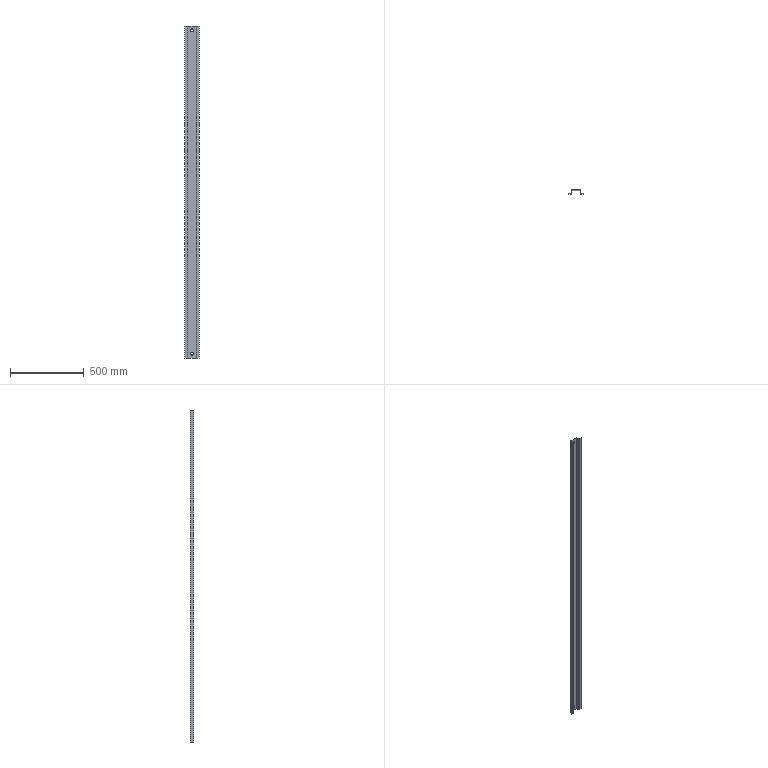Part | 1 solid | 42 faces | box 98.4 x 25 x 2251 mm | volume 259526 mm3 | plane 30 | cylinder 12 | commonest cylinder face diameters 2 x4 3.6 x4 20 x4
STEP:
#1=CARTESIAN_POINT('',(10.,-0.8,-1095.5));
#2=VERTEX_POINT('',#1);
#3=CARTESIAN_POINT('',(-10.,-0.8,-1095.5));
#4=VERTEX_POINT('',#3);
#5=CARTESIAN_POINT('',(0.,-0.8,-1095.5));
#6=DIRECTION('',(0.,1.,0.));
#7=DIRECTION('',(-1.,0.,0.));
#8=AXIS2_PLACEMENT_3D('',#5,#6,#7);
#9=CIRCLE('',#8,10.);
#10=EDGE_CURVE('',#2,#4,#9,.T.);
#11=ORIENTED_EDGE('',*,*,#10,.F.);
#12=CARTESIAN_POINT('',(10.,0.,-1095.5));
#13=VERTEX_POINT('',#12);
#14=CARTESIAN_POINT('',(10.,-10.,-1095.5));
#15=DIRECTION('',(0.,1.,0.));
#16=VECTOR('',#15,1000.);
#17=LINE('',#14,#16);
#18=EDGE_CURVE('',#2,#13,#17,.T.);
#19=ORIENTED_EDGE('',*,*,#18,.T.);
#20=CARTESIAN_POINT('',(-10.,0.,-1095.5));
#21=VERTEX_POINT('',#20);
#22=CARTESIAN_POINT('',(0.,0.,-1095.5));
#23=DIRECTION('',(0.,1.,0.));
#24=DIRECTION('',(-1.,0.,0.));
#25=AXIS2_PLACEMENT_3D('',#22,#23,#24);
#26=CIRCLE('',#25,10.);
#27=EDGE_CURVE('',#13,#21,#26,.T.);
#28=ORIENTED_EDGE('',*,*,#27,.T.);
#29=CARTESIAN_POINT('',(-10.,-10.,-1095.5));
#30=DIRECTION('',(0.,1.,0.));
#31=VECTOR('',#30,1000.);
#32=LINE('',#29,#31);
#33=EDGE_CURVE('',#4,#21,#32,.T.);
#34=ORIENTED_EDGE('',*,*,#33,.F.);
#35=EDGE_LOOP('',(#11,#19,#28,#34));
#36=FACE_OUTER_BOUND('',#35,.T.);
#37=CARTESIAN_POINT('',(0.,-10.,-1095.5));
#38=DIRECTION('',(0.,1.,0.));
#39=DIRECTION('',(-1.,0.,0.));
#40=AXIS2_PLACEMENT_3D('',#37,#38,#39);
#41=CYLINDRICAL_SURFACE('',#40,10.);
#42=ADVANCED_FACE('',(#36),#41,.F.);
#43=CARTESIAN_POINT('',(10.,-0.8,1095.5));
#44=VERTEX_POINT('',#43);
#45=CARTESIAN_POINT('',(-10.,-0.8,1095.5));
#46=VERTEX_POINT('',#45);
#47=CARTESIAN_POINT('',(0.,-0.8,1095.5));
#48=DIRECTION('',(0.,1.,0.));
#49=DIRECTION('',(-1.,0.,0.));
#50=AXIS2_PLACEMENT_3D('',#47,#48,#49);
#51=CIRCLE('',#50,10.);
#52=EDGE_CURVE('',#44,#46,#51,.T.);
#53=ORIENTED_EDGE('',*,*,#52,.F.);
#54=CARTESIAN_POINT('',(10.,0.,1095.5));
#55=VERTEX_POINT('',#54);
#56=CARTESIAN_POINT('',(10.,-10.,1095.5));
#57=DIRECTION('',(0.,1.,0.));
#58=VECTOR('',#57,1000.);
#59=LINE('',#56,#58);
#60=EDGE_CURVE('',#44,#55,#59,.T.);
#61=ORIENTED_EDGE('',*,*,#60,.T.);
#62=CARTESIAN_POINT('',(-10.,0.,1095.5));
#63=VERTEX_POINT('',#62);
#64=CARTESIAN_POINT('',(0.,0.,1095.5));
#65=DIRECTION('',(0.,1.,0.));
#66=DIRECTION('',(1.,0.,0.));
#67=AXIS2_PLACEMENT_3D('',#64,#65,#66);
#68=CIRCLE('',#67,10.);
#69=EDGE_CURVE('',#55,#63,#68,.T.);
#70=ORIENTED_EDGE('',*,*,#69,.T.);
#71=CARTESIAN_POINT('',(-10.,-10.,1095.5));
#72=DIRECTION('',(0.,1.,0.));
#73=VECTOR('',#72,1000.);
#74=LINE('',#71,#73);
#75=EDGE_CURVE('',#46,#63,#74,.T.);
#76=ORIENTED_EDGE('',*,*,#75,.F.);
#77=EDGE_LOOP('',(#53,#61,#70,#76));
#78=FACE_OUTER_BOUND('',#77,.T.);
#79=CARTESIAN_POINT('',(0.,-10.,1095.5));
#80=DIRECTION('',(0.,1.,0.));
#81=DIRECTION('',(-1.,0.,0.));
#82=AXIS2_PLACEMENT_3D('',#79,#80,#81);
#83=CYLINDRICAL_SURFACE('',#82,10.);
#84=ADVANCED_FACE('',(#78),#83,.F.);
#85=CARTESIAN_POINT('',(29.2,-23.2,-1125.5));
#86=VERTEX_POINT('',#85);
#87=CARTESIAN_POINT('',(29.2,-23.2,1125.5));
#88=VERTEX_POINT('',#87);
#89=CARTESIAN_POINT('',(29.2,-23.2,-1125.5));
#90=DIRECTION('',(0.,0.,1.));
#91=VECTOR('',#90,1000.);
#92=LINE('',#89,#91);
#93=EDGE_CURVE('',#86,#88,#92,.T.);
#94=ORIENTED_EDGE('',*,*,#93,.T.);
#95=CARTESIAN_POINT('',(29.2,-1.8,1125.5));
#96=VERTEX_POINT('',#95);
#97=CARTESIAN_POINT('',(29.2,0.,1125.5));
#98=DIRECTION('',(0.,-1.,0.));
#99=VECTOR('',#98,1000.);
#100=LINE('',#97,#99);
#101=EDGE_CURVE('',#96,#88,#100,.T.);
#102=ORIENTED_EDGE('',*,*,#101,.F.);
#103=CARTESIAN_POINT('',(29.2,-1.8,-1125.5));
#104=VERTEX_POINT('',#103);
#105=CARTESIAN_POINT('',(29.2,-1.8,1125.5));
#106=DIRECTION('',(0.,0.,-1.));
#107=VECTOR('',#106,1000.);
#108=LINE('',#105,#107);
#109=EDGE_CURVE('',#96,#104,#108,.T.);
#110=ORIENTED_EDGE('',*,*,#109,.T.);
#111=CARTESIAN_POINT('',(29.2,0.,-1125.5));
#112=DIRECTION('',(0.,-1.,0.));
#113=VECTOR('',#112,1000.);
#114=LINE('',#111,#113);
#115=EDGE_CURVE('',#104,#86,#114,.T.);
#116=ORIENTED_EDGE('',*,*,#115,.T.);
#117=EDGE_LOOP('',(#94,#102,#110,#116));
#118=FACE_OUTER_BOUND('',#117,.T.);
#119=CARTESIAN_POINT('',(29.2,0.,1125.5));
#120=DIRECTION('',(1.,0.,0.));
#121=DIRECTION('',(0.,1.,0.));
#122=AXIS2_PLACEMENT_3D('',#119,#120,#121);
#123=PLANE('',#122);
#124=ADVANCED_FACE('',(#118),#123,.F.);
#125=CARTESIAN_POINT('',(30.,-1.8,1125.5));
#126=VERTEX_POINT('',#125);
#127=CARTESIAN_POINT('',(30.,-23.2,1125.5));
#128=VERTEX_POINT('',#127);
#129=CARTESIAN_POINT('',(30.,0.,1125.5));
#130=DIRECTION('',(0.,-1.,0.));
#131=VECTOR('',#130,1000.);
#132=LINE('',#129,#131);
#133=EDGE_CURVE('',#126,#128,#132,.T.);
#134=ORIENTED_EDGE('',*,*,#133,.T.);
#135=CARTESIAN_POINT('',(30.,-23.2,-1125.5));
#136=VERTEX_POINT('',#135);
#137=CARTESIAN_POINT('',(30.,-23.2,-1125.5));
#138=DIRECTION('',(0.,0.,1.));
#139=VECTOR('',#138,1000.);
#140=LINE('',#137,#139);
#141=EDGE_CURVE('',#136,#128,#140,.T.);
#142=ORIENTED_EDGE('',*,*,#141,.F.);
#143=CARTESIAN_POINT('',(30.,-1.8,-1125.5));
#144=VERTEX_POINT('',#143);
#145=CARTESIAN_POINT('',(30.,0.,-1125.5));
#146=DIRECTION('',(0.,-1.,0.));
#147=VECTOR('',#146,1000.);
#148=LINE('',#145,#147);
#149=EDGE_CURVE('',#144,#136,#148,.T.);
#150=ORIENTED_EDGE('',*,*,#149,.F.);
#151=CARTESIAN_POINT('',(30.,-1.8,1125.5));
#152=DIRECTION('',(0.,0.,-1.));
#153=VECTOR('',#152,1000.);
#154=LINE('',#151,#153);
#155=EDGE_CURVE('',#126,#144,#154,.T.);
#156=ORIENTED_EDGE('',*,*,#155,.F.);
#157=EDGE_LOOP('',(#134,#142,#150,#156));
#158=FACE_OUTER_BOUND('',#157,.T.);
#159=CARTESIAN_POINT('',(30.,0.,1125.5));
#160=DIRECTION('',(1.,0.,0.));
#161=DIRECTION('',(0.,1.,0.));
#162=AXIS2_PLACEMENT_3D('',#159,#160,#161);
#163=PLANE('',#162);
#164=ADVANCED_FACE('',(#158),#163,.T.);
#165=CARTESIAN_POINT('',(30.,-23.2,-1125.5));
#166=DIRECTION('',(-1.,0.,0.));
#167=VECTOR('',#166,1000.);
#168=LINE('',#165,#167);
#169=EDGE_CURVE('',#136,#86,#168,.T.);
#170=ORIENTED_EDGE('',*,*,#169,.T.);
#171=ORIENTED_EDGE('',*,*,#115,.F.);
#172=CARTESIAN_POINT('',(29.2,-1.8,-1125.5));
#173=DIRECTION('',(1.,0.,0.));
#174=VECTOR('',#173,1000.);
#175=LINE('',#172,#174);
#176=EDGE_CURVE('',#104,#144,#175,.T.);
#177=ORIENTED_EDGE('',*,*,#176,.T.);
#178=ORIENTED_EDGE('',*,*,#149,.T.);
#179=EDGE_LOOP('',(#170,#171,#177,#178));
#180=FACE_OUTER_BOUND('',#179,.T.);
#181=CARTESIAN_POINT('',(28.2,-1.8,-1125.5));
#182=DIRECTION('',(0.,0.,1.));
#183=DIRECTION('',(1.,0.,0.));
#184=AXIS2_PLACEMENT_3D('',#181,#182,#183);
#185=PLANE('',#184);
#186=ADVANCED_FACE('',(#180),#185,.F.);
#187=CARTESIAN_POINT('',(-30.,-23.2,-1125.5));
#188=VERTEX_POINT('',#187);
#189=CARTESIAN_POINT('',(-30.,-1.8,-1125.5));
#190=VERTEX_POINT('',#189);
#191=CARTESIAN_POINT('',(-30.,-25.,-1125.5));
#192=DIRECTION('',(0.,1.,0.));
#193=VECTOR('',#192,1000.);
#194=LINE('',#191,#193);
#195=EDGE_CURVE('',#188,#190,#194,.T.);
#196=ORIENTED_EDGE('',*,*,#195,.F.);
#197=CARTESIAN_POINT('',(-30.,-23.2,1125.5));
#198=VERTEX_POINT('',#197);
#199=CARTESIAN_POINT('',(-30.,-23.2,1125.5));
#200=DIRECTION('',(0.,0.,-1.));
#201=VECTOR('',#200,1000.);
#202=LINE('',#199,#201);
#203=EDGE_CURVE('',#198,#188,#202,.T.);
#204=ORIENTED_EDGE('',*,*,#203,.F.);
#205=CARTESIAN_POINT('',(-30.,-1.8,1125.5));
#206=VERTEX_POINT('',#205);
#207=CARTESIAN_POINT('',(-30.,-25.,1125.5));
#208=DIRECTION('',(0.,1.,0.));
#209=VECTOR('',#208,1000.);
#210=LINE('',#207,#209);
#211=EDGE_CURVE('',#198,#206,#210,.T.);
#212=ORIENTED_EDGE('',*,*,#211,.T.);
#213=CARTESIAN_POINT('',(-30.,-1.8,1125.5));
#214=DIRECTION('',(0.,0.,-1.));
#215=VECTOR('',#214,1000.);
#216=LINE('',#213,#215);
#217=EDGE_CURVE('',#206,#190,#216,.T.);
#218=ORIENTED_EDGE('',*,*,#217,.T.);
#219=EDGE_LOOP('',(#196,#204,#212,#218));
#220=FACE_OUTER_BOUND('',#219,.T.);
#221=CARTESIAN_POINT('',(-30.,-25.,1125.5));
#222=DIRECTION('',(-1.,0.,0.));
#223=DIRECTION('',(0.,0.,1.));
#224=AXIS2_PLACEMENT_3D('',#221,#222,#223);
#225=PLANE('',#224);
#226=ADVANCED_FACE('',(#220),#225,.T.);
#227=CARTESIAN_POINT('',(-29.2,-23.2,1125.5));
#228=VERTEX_POINT('',#227);
#229=CARTESIAN_POINT('',(-29.2,-23.2,-1125.5));
#230=VERTEX_POINT('',#229);
#231=CARTESIAN_POINT('',(-29.2,-23.2,1125.5));
#232=DIRECTION('',(0.,0.,-1.));
#233=VECTOR('',#232,1000.);
#234=LINE('',#231,#233);
#235=EDGE_CURVE('',#228,#230,#234,.T.);
#236=ORIENTED_EDGE('',*,*,#235,.T.);
#237=CARTESIAN_POINT('',(-29.2,-1.8,-1125.5));
#238=VERTEX_POINT('',#237);
#239=CARTESIAN_POINT('',(-29.2,-25.,-1125.5));
#240=DIRECTION('',(0.,1.,0.));
#241=VECTOR('',#240,1000.);
#242=LINE('',#239,#241);
#243=EDGE_CURVE('',#230,#238,#242,.T.);
#244=ORIENTED_EDGE('',*,*,#243,.T.);
#245=CARTESIAN_POINT('',(-29.2,-1.8,1125.5));
#246=VERTEX_POINT('',#245);
#247=CARTESIAN_POINT('',(-29.2,-1.8,1125.5));
#248=DIRECTION('',(0.,0.,-1.));
#249=VECTOR('',#248,1000.);
#250=LINE('',#247,#249);
#251=EDGE_CURVE('',#246,#238,#250,.T.);
#252=ORIENTED_EDGE('',*,*,#251,.F.);
#253=CARTESIAN_POINT('',(-29.2,-25.,1125.5));
#254=DIRECTION('',(0.,1.,0.));
#255=VECTOR('',#254,1000.);
#256=LINE('',#253,#255);
#257=EDGE_CURVE('',#228,#246,#256,.T.);
#258=ORIENTED_EDGE('',*,*,#257,.F.);
#259=EDGE_LOOP('',(#236,#244,#252,#258));
#260=FACE_OUTER_BOUND('',#259,.T.);
#261=CARTESIAN_POINT('',(-29.2,-25.,1125.5));
#262=DIRECTION('',(-1.,0.,0.));
#263=DIRECTION('',(0.,0.,1.));
#264=AXIS2_PLACEMENT_3D('',#261,#262,#263);
#265=PLANE('',#264);
#266=ADVANCED_FACE('',(#260),#265,.F.);
#267=ORIENTED_EDGE('',*,*,#211,.F.);
#268=CARTESIAN_POINT('',(-30.,-23.2,1125.5));
#269=DIRECTION('',(1.,0.,0.));
#270=VECTOR('',#269,1000.);
#271=LINE('',#268,#270);
#272=EDGE_CURVE('',#198,#228,#271,.T.);
#273=ORIENTED_EDGE('',*,*,#272,.T.);
#274=ORIENTED_EDGE('',*,*,#257,.T.);
#275=CARTESIAN_POINT('',(-29.2,-1.8,1125.5));
#276=DIRECTION('',(-1.,0.,0.));
#277=VECTOR('',#276,1000.);
#278=LINE('',#275,#277);
#279=EDGE_CURVE('',#246,#206,#278,.T.);
#280=ORIENTED_EDGE('',*,*,#279,.T.);
#281=EDGE_LOOP('',(#267,#273,#274,#280));
#282=FACE_OUTER_BOUND('',#281,.T.);
#283=CARTESIAN_POINT('',(28.2,-1.8,1125.5));
#284=DIRECTION('',(0.,0.,1.));
#285=DIRECTION('',(1.,0.,0.));
#286=AXIS2_PLACEMENT_3D('',#283,#284,#285);
#287=PLANE('',#286);
#288=ADVANCED_FACE('',(#282),#287,.T.);
#289=CARTESIAN_POINT('',(-28.2,0.,1125.5));
#290=VERTEX_POINT('',#289);
#291=CARTESIAN_POINT('',(-28.2,-0.8,1125.5));
#292=VERTEX_POINT('',#291);
#293=CARTESIAN_POINT('',(-28.2,0.,1125.5));
#294=DIRECTION('',(0.,-1.,0.));
#295=VECTOR('',#294,1000.);
#296=LINE('',#293,#295);
#297=EDGE_CURVE('',#290,#292,#296,.T.);
#298=ORIENTED_EDGE('',*,*,#297,.F.);
#299=CARTESIAN_POINT('',(-28.2,-1.8,1125.5));
#300=DIRECTION('',(0.,0.,-1.));
#301=DIRECTION('',(1.,0.,0.));
#302=AXIS2_PLACEMENT_3D('',#299,#300,#301);
#303=CIRCLE('',#302,1.8);
#304=EDGE_CURVE('',#206,#290,#303,.T.);
#305=ORIENTED_EDGE('',*,*,#304,.F.);
#306=ORIENTED_EDGE('',*,*,#279,.F.);
#307=CARTESIAN_POINT('',(-28.2,-1.8,1125.5));
#308=DIRECTION('',(0.,0.,-1.));
#309=DIRECTION('',(1.,0.,0.));
#310=AXIS2_PLACEMENT_3D('',#307,#308,#309);
#311=CIRCLE('',#310,1.);
#312=EDGE_CURVE('',#246,#292,#311,.T.);
#313=ORIENTED_EDGE('',*,*,#312,.T.);
#314=EDGE_LOOP('',(#298,#305,#306,#313));
#315=FACE_OUTER_BOUND('',#314,.T.);
#316=CARTESIAN_POINT('',(-28.2,0.,1125.5));
#317=DIRECTION('',(0.,0.,1.));
#318=DIRECTION('',(1.,0.,0.));
#319=AXIS2_PLACEMENT_3D('',#316,#317,#318);
#320=PLANE('',#319);
#321=ADVANCED_FACE('',(#315),#320,.T.);
#322=CARTESIAN_POINT('',(28.2,0.,1125.5));
#323=VERTEX_POINT('',#322);
#324=CARTESIAN_POINT('',(-30.,0.,1125.5));
#325=DIRECTION('',(1.,0.,0.));
#326=VECTOR('',#325,1000.);
#327=LINE('',#324,#326);
#328=EDGE_CURVE('',#290,#323,#327,.T.);
#329=ORIENTED_EDGE('',*,*,#328,.F.);
#330=ORIENTED_EDGE('',*,*,#297,.T.);
#331=CARTESIAN_POINT('',(28.2,-0.8,1125.5));
#332=VERTEX_POINT('',#331);
#333=CARTESIAN_POINT('',(-30.,-0.8,1125.5));
#334=DIRECTION('',(1.,0.,0.));
#335=VECTOR('',#334,1000.);
#336=LINE('',#333,#335);
#337=EDGE_CURVE('',#292,#332,#336,.T.);
#338=ORIENTED_EDGE('',*,*,#337,.T.);
#339=CARTESIAN_POINT('',(28.2,-0.8,1125.5));
#340=DIRECTION('',(0.,1.,0.));
#341=VECTOR('',#340,1000.);
#342=LINE('',#339,#341);
#343=EDGE_CURVE('',#332,#323,#342,.T.);
#344=ORIENTED_EDGE('',*,*,#343,.T.);
#345=EDGE_LOOP('',(#329,#330,#338,#344));
#346=FACE_OUTER_BOUND('',#345,.T.);
#347=CARTESIAN_POINT('',(-29.2,-1.8,1125.5));
#348=DIRECTION('',(0.,0.,1.));
#349=DIRECTION('',(1.,0.,0.));
#350=AXIS2_PLACEMENT_3D('',#347,#348,#349);
#351=PLANE('',#350);
#352=ADVANCED_FACE('',(#346),#351,.T.);
#353=CARTESIAN_POINT('',(-30.,-1.8,-1125.5));
#354=DIRECTION('',(1.,0.,0.));
#355=VECTOR('',#354,1000.);
#356=LINE('',#353,#355);
#357=EDGE_CURVE('',#190,#238,#356,.T.);
#358=ORIENTED_EDGE('',*,*,#357,.F.);
#359=CARTESIAN_POINT('',(-28.2,0.,-1125.5));
#360=VERTEX_POINT('',#359);
#361=CARTESIAN_POINT('',(-28.2,-1.8,-1125.5));
#362=DIRECTION('',(0.,0.,-1.));
#363=DIRECTION('',(1.,0.,0.));
#364=AXIS2_PLACEMENT_3D('',#361,#362,#363);
#365=CIRCLE('',#364,1.8);
#366=EDGE_CURVE('',#190,#360,#365,.T.);
#367=ORIENTED_EDGE('',*,*,#366,.T.);
#368=CARTESIAN_POINT('',(-28.2,-0.8,-1125.5));
#369=VERTEX_POINT('',#368);
#370=CARTESIAN_POINT('',(-28.2,-0.8,-1125.5));
#371=DIRECTION('',(0.,1.,0.));
#372=VECTOR('',#371,1000.);
#373=LINE('',#370,#372);
#374=EDGE_CURVE('',#369,#360,#373,.T.);
#375=ORIENTED_EDGE('',*,*,#374,.F.);
#376=CARTESIAN_POINT('',(-28.2,-1.8,-1125.5));
#377=DIRECTION('',(0.,0.,-1.));
#378=DIRECTION('',(1.,0.,0.));
#379=AXIS2_PLACEMENT_3D('',#376,#377,#378);
#380=CIRCLE('',#379,1.);
#381=EDGE_CURVE('',#238,#369,#380,.T.);
#382=ORIENTED_EDGE('',*,*,#381,.F.);
#383=EDGE_LOOP('',(#358,#367,#375,#382));
#384=FACE_OUTER_BOUND('',#383,.T.);
#385=CARTESIAN_POINT('',(-30.,-1.8,-1125.5));
#386=DIRECTION('',(0.,0.,-1.));
#387=DIRECTION('',(-1.,0.,0.));
#388=AXIS2_PLACEMENT_3D('',#385,#386,#387);
#389=PLANE('',#388);
#390=ADVANCED_FACE('',(#384),#389,.T.);
#391=CARTESIAN_POINT('',(-30.,-23.2,-1125.5));
#392=DIRECTION('',(1.,0.,0.));
#393=VECTOR('',#392,1000.);
#394=LINE('',#391,#393);
#395=EDGE_CURVE('',#188,#230,#394,.T.);
#396=ORIENTED_EDGE('',*,*,#395,.F.);
#397=ORIENTED_EDGE('',*,*,#195,.T.);
#398=ORIENTED_EDGE('',*,*,#357,.T.);
#399=ORIENTED_EDGE('',*,*,#243,.F.);
#400=EDGE_LOOP('',(#396,#397,#398,#399));
#401=FACE_OUTER_BOUND('',#400,.T.);
#402=CARTESIAN_POINT('',(-28.2,-0.8,-1125.5));
#403=DIRECTION('',(0.,0.,-1.));
#404=DIRECTION('',(-1.,0.,0.));
#405=AXIS2_PLACEMENT_3D('',#402,#403,#404);
#406=PLANE('',#405);
#407=ADVANCED_FACE('',(#401),#406,.T.);
#408=CARTESIAN_POINT('',(30.,-1.8,1125.5));
#409=DIRECTION('',(-1.,0.,0.));
#410=VECTOR('',#409,1000.);
#411=LINE('',#408,#410);
#412=EDGE_CURVE('',#126,#96,#411,.T.);
#413=ORIENTED_EDGE('',*,*,#412,.F.);
#414=CARTESIAN_POINT('',(28.2,-1.8,1125.5));
#415=DIRECTION('',(0.,0.,-1.));
#416=DIRECTION('',(1.,0.,0.));
#417=AXIS2_PLACEMENT_3D('',#414,#415,#416);
#418=CIRCLE('',#417,1.8);
#419=EDGE_CURVE('',#323,#126,#418,.T.);
#420=ORIENTED_EDGE('',*,*,#419,.F.);
#421=ORIENTED_EDGE('',*,*,#343,.F.);
#422=CARTESIAN_POINT('',(28.2,-1.8,1125.5));
#423=DIRECTION('',(0.,0.,-1.));
#424=DIRECTION('',(1.,0.,0.));
#425=AXIS2_PLACEMENT_3D('',#422,#423,#424);
#426=CIRCLE('',#425,1.);
#427=EDGE_CURVE('',#332,#96,#426,.T.);
#428=ORIENTED_EDGE('',*,*,#427,.T.);
#429=EDGE_LOOP('',(#413,#420,#421,#428));
#430=FACE_OUTER_BOUND('',#429,.T.);
#431=CARTESIAN_POINT('',(30.,-1.8,1125.5));
#432=DIRECTION('',(0.,0.,1.));
#433=DIRECTION('',(1.,0.,0.));
#434=AXIS2_PLACEMENT_3D('',#431,#432,#433);
#435=PLANE('',#434);
#436=ADVANCED_FACE('',(#430),#435,.T.);
#437=CARTESIAN_POINT('',(30.,-23.2,1125.5));
#438=DIRECTION('',(-1.,0.,0.));
#439=VECTOR('',#438,1000.);
#440=LINE('',#437,#439);
#441=EDGE_CURVE('',#128,#88,#440,.T.);
#442=ORIENTED_EDGE('',*,*,#441,.F.);
#443=ORIENTED_EDGE('',*,*,#133,.F.);
#444=ORIENTED_EDGE('',*,*,#412,.T.);
#445=ORIENTED_EDGE('',*,*,#101,.T.);
#446=EDGE_LOOP('',(#442,#443,#444,#445));
#447=FACE_OUTER_BOUND('',#446,.T.);
#448=CARTESIAN_POINT('',(28.2,-0.8,1125.5));
#449=DIRECTION('',(0.,0.,1.));
#450=DIRECTION('',(1.,0.,0.));
#451=AXIS2_PLACEMENT_3D('',#448,#449,#450);
#452=PLANE('',#451);
#453=ADVANCED_FACE('',(#447),#452,.T.);
#454=CARTESIAN_POINT('',(28.2,0.,-1125.5));
#455=VERTEX_POINT('',#454);
#456=CARTESIAN_POINT('',(28.2,-0.8,-1125.5));
#457=VERTEX_POINT('',#456);
#458=CARTESIAN_POINT('',(28.2,0.,-1125.5));
#459=DIRECTION('',(0.,-1.,0.));
#460=VECTOR('',#459,1000.);
#461=LINE('',#458,#460);
#462=EDGE_CURVE('',#455,#457,#461,.T.);
#463=ORIENTED_EDGE('',*,*,#462,.F.);
#464=CARTESIAN_POINT('',(28.2,-1.8,-1125.5));
#465=DIRECTION('',(0.,0.,-1.));
#466=DIRECTION('',(1.,0.,0.));
#467=AXIS2_PLACEMENT_3D('',#464,#465,#466);
#468=CIRCLE('',#467,1.8);
#469=EDGE_CURVE('',#455,#144,#468,.T.);
#470=ORIENTED_EDGE('',*,*,#469,.T.);
#471=ORIENTED_EDGE('',*,*,#176,.F.);
#472=CARTESIAN_POINT('',(28.2,-1.8,-1125.5));
#473=DIRECTION('',(0.,0.,-1.));
#474=DIRECTION('',(1.,0.,0.));
#475=AXIS2_PLACEMENT_3D('',#472,#473,#474);
#476=CIRCLE('',#475,1.);
#477=EDGE_CURVE('',#457,#104,#476,.T.);
#478=ORIENTED_EDGE('',*,*,#477,.F.);
#479=EDGE_LOOP('',(#463,#470,#471,#478));
#480=FACE_OUTER_BOUND('',#479,.T.);
#481=CARTESIAN_POINT('',(28.2,0.,-1125.5));
#482=DIRECTION('',(0.,0.,-1.));
#483=DIRECTION('',(-1.,0.,0.));
#484=AXIS2_PLACEMENT_3D('',#481,#482,#483);
#485=PLANE('',#484);
#486=ADVANCED_FACE('',(#480),#485,.T.);
#487=CARTESIAN_POINT('',(-30.,0.,-1125.5));
#488=DIRECTION('',(1.,0.,0.));
#489=VECTOR('',#488,1000.);
#490=LINE('',#487,#489);
#491=EDGE_CURVE('',#360,#455,#490,.T.);
#492=ORIENTED_EDGE('',*,*,#491,.T.);
#493=ORIENTED_EDGE('',*,*,#462,.T.);
#494=CARTESIAN_POINT('',(-30.,-0.8,-1125.5));
#495=DIRECTION('',(1.,0.,0.));
#496=VECTOR('',#495,1000.);
#497=LINE('',#494,#496);
#498=EDGE_CURVE('',#369,#457,#497,.T.);
#499=ORIENTED_EDGE('',*,*,#498,.F.);
#500=ORIENTED_EDGE('',*,*,#374,.T.);
#501=EDGE_LOOP('',(#492,#493,#499,#500));
#502=FACE_OUTER_BOUND('',#501,.T.);
#503=CARTESIAN_POINT('',(29.2,-1.8,-1125.5));
#504=DIRECTION('',(0.,0.,-1.));
#505=DIRECTION('',(-1.,0.,0.));
#506=AXIS2_PLACEMENT_3D('',#503,#504,#505);
#507=PLANE('',#506);
#508=ADVANCED_FACE('',(#502),#507,.T.);
#509=ORIENTED_EDGE('',*,*,#469,.F.);
#510=CARTESIAN_POINT('',(28.2,0.,1125.5));
#511=DIRECTION('',(0.,0.,-1.));
#512=VECTOR('',#511,1000.);
#513=LINE('',#510,#512);
#514=EDGE_CURVE('',#323,#455,#513,.T.);
#515=ORIENTED_EDGE('',*,*,#514,.F.);
#516=ORIENTED_EDGE('',*,*,#419,.T.);
#517=ORIENTED_EDGE('',*,*,#155,.T.);
#518=EDGE_LOOP('',(#509,#515,#516,#517));
#519=FACE_OUTER_BOUND('',#518,.T.);
#520=CARTESIAN_POINT('',(28.2,-1.8,1125.5));
#521=DIRECTION('',(0.,0.,-1.));
#522=DIRECTION('',(-1.,0.,0.));
#523=AXIS2_PLACEMENT_3D('',#520,#521,#522);
#524=CYLINDRICAL_SURFACE('',#523,1.8);
#525=ADVANCED_FACE('',(#519),#524,.T.);
#526=CARTESIAN_POINT('',(0.,0.,-1095.5));
#527=DIRECTION('',(0.,1.,0.));
#528=DIRECTION('',(-1.,0.,0.));
#529=AXIS2_PLACEMENT_3D('',#526,#527,#528);
#530=CIRCLE('',#529,10.);
#531=EDGE_CURVE('',#21,#13,#530,.T.);
#532=ORIENTED_EDGE('',*,*,#531,.F.);
#533=ORIENTED_EDGE('',*,*,#27,.F.);
#534=EDGE_LOOP('',(#532,#533));
#535=FACE_BOUND('',#534,.T.);
#536=CARTESIAN_POINT('',(0.,0.,1095.5));
#537=DIRECTION('',(0.,1.,0.));
#538=DIRECTION('',(1.,0.,0.));
#539=AXIS2_PLACEMENT_3D('',#536,#537,#538);
#540=CIRCLE('',#539,10.);
#541=EDGE_CURVE('',#63,#55,#540,.T.);
#542=ORIENTED_EDGE('',*,*,#541,.F.);
#543=ORIENTED_EDGE('',*,*,#69,.F.);
#544=EDGE_LOOP('',(#542,#543));
#545=FACE_BOUND('',#544,.T.);
#546=ORIENTED_EDGE('',*,*,#491,.F.);
#547=CARTESIAN_POINT('',(-28.2,0.,1125.5));
#548=DIRECTION('',(0.,0.,-1.));
#549=VECTOR('',#548,1000.);
#550=LINE('',#547,#549);
#551=EDGE_CURVE('',#290,#360,#550,.T.);
#552=ORIENTED_EDGE('',*,*,#551,.F.);
#553=ORIENTED_EDGE('',*,*,#328,.T.);
#554=ORIENTED_EDGE('',*,*,#514,.T.);
#555=EDGE_LOOP('',(#546,#552,#553,#554));
#556=FACE_OUTER_BOUND('',#555,.T.);
#557=CARTESIAN_POINT('',(-30.,0.,1125.5));
#558=DIRECTION('',(0.,1.,0.));
#559=DIRECTION('',(-1.,0.,0.));
#560=AXIS2_PLACEMENT_3D('',#557,#558,#559);
#561=PLANE('',#560);
#562=ADVANCED_FACE('',(#535,#545,#556),#561,.T.);
#563=ORIENTED_EDGE('',*,*,#366,.F.);
#564=ORIENTED_EDGE('',*,*,#217,.F.);
#565=ORIENTED_EDGE('',*,*,#304,.T.);
#566=ORIENTED_EDGE('',*,*,#551,.T.);
#567=EDGE_LOOP('',(#563,#564,#565,#566));
#568=FACE_OUTER_BOUND('',#567,.T.);
#569=CARTESIAN_POINT('',(-28.2,-1.8,1125.5));
#570=DIRECTION('',(0.,0.,-1.));
#571=DIRECTION('',(-1.,0.,0.));
#572=AXIS2_PLACEMENT_3D('',#569,#570,#571);
#573=CYLINDRICAL_SURFACE('',#572,1.8);
#574=ADVANCED_FACE('',(#568),#573,.T.);
#575=ORIENTED_EDGE('',*,*,#381,.T.);
#576=CARTESIAN_POINT('',(-28.2,-0.8,1125.5));
#577=DIRECTION('',(0.,0.,-1.));
#578=VECTOR('',#577,1000.);
#579=LINE('',#576,#578);
#580=EDGE_CURVE('',#292,#369,#579,.T.);
#581=ORIENTED_EDGE('',*,*,#580,.F.);
#582=ORIENTED_EDGE('',*,*,#312,.F.);
#583=ORIENTED_EDGE('',*,*,#251,.T.);
#584=EDGE_LOOP('',(#575,#581,#582,#583));
#585=FACE_OUTER_BOUND('',#584,.T.);
#586=CARTESIAN_POINT('',(-28.2,-1.8,1125.5));
#587=DIRECTION('',(0.,0.,-1.));
#588=DIRECTION('',(-1.,0.,0.));
#589=AXIS2_PLACEMENT_3D('',#586,#587,#588);
#590=CYLINDRICAL_SURFACE('',#589,1.);
#591=ADVANCED_FACE('',(#585),#590,.F.);
#592=CARTESIAN_POINT('',(0.,-0.8,-1095.5));
#593=DIRECTION('',(0.,1.,0.));
#594=DIRECTION('',(-1.,0.,0.));
#595=AXIS2_PLACEMENT_3D('',#592,#593,#594);
#596=CIRCLE('',#595,10.);
#597=EDGE_CURVE('',#4,#2,#596,.T.);
#598=ORIENTED_EDGE('',*,*,#597,.T.);
#599=ORIENTED_EDGE('',*,*,#10,.T.);
#600=EDGE_LOOP('',(#598,#599));
#601=FACE_BOUND('',#600,.T.);
#602=CARTESIAN_POINT('',(0.,-0.8,1095.5));
#603=DIRECTION('',(0.,1.,0.));
#604=DIRECTION('',(-1.,0.,0.));
#605=AXIS2_PLACEMENT_3D('',#602,#603,#604);
#606=CIRCLE('',#605,10.);
#607=EDGE_CURVE('',#46,#44,#606,.T.);
#608=ORIENTED_EDGE('',*,*,#607,.T.);
#609=ORIENTED_EDGE('',*,*,#52,.T.);
#610=EDGE_LOOP('',(#608,#609));
#611=FACE_BOUND('',#610,.T.);
#612=ORIENTED_EDGE('',*,*,#498,.T.);
#613=CARTESIAN_POINT('',(28.2,-0.8,1125.5));
#614=DIRECTION('',(0.,0.,-1.));
#615=VECTOR('',#614,1000.);
#616=LINE('',#613,#615);
#617=EDGE_CURVE('',#332,#457,#616,.T.);
#618=ORIENTED_EDGE('',*,*,#617,.F.);
#619=ORIENTED_EDGE('',*,*,#337,.F.);
#620=ORIENTED_EDGE('',*,*,#580,.T.);
#621=EDGE_LOOP('',(#612,#618,#619,#620));
#622=FACE_OUTER_BOUND('',#621,.T.);
#623=CARTESIAN_POINT('',(-30.,-0.8,1125.5));
#624=DIRECTION('',(0.,1.,0.));
#625=DIRECTION('',(-1.,0.,0.));
#626=AXIS2_PLACEMENT_3D('',#623,#624,#625);
#627=PLANE('',#626);
#628=ADVANCED_FACE('',(#601,#611,#622),#627,.F.);
#629=ORIENTED_EDGE('',*,*,#477,.T.);
#630=ORIENTED_EDGE('',*,*,#109,.F.);
#631=ORIENTED_EDGE('',*,*,#427,.F.);
#632=ORIENTED_EDGE('',*,*,#617,.T.);
#633=EDGE_LOOP('',(#629,#630,#631,#632));
#634=FACE_OUTER_BOUND('',#633,.T.);
#635=CARTESIAN_POINT('',(28.2,-1.8,1125.5));
#636=DIRECTION('',(0.,0.,-1.));
#637=DIRECTION('',(-1.,0.,0.));
#638=AXIS2_PLACEMENT_3D('',#635,#636,#637);
#639=CYLINDRICAL_SURFACE('',#638,1.);
#640=ADVANCED_FACE('',(#634),#639,.F.);
#641=CARTESIAN_POINT('',(-31.,-24.2,-1125.5));
#642=VERTEX_POINT('',#641);
#643=CARTESIAN_POINT('',(-31.,-25.,-1125.5));
#644=VERTEX_POINT('',#643);
#645=CARTESIAN_POINT('',(-31.,-25.,-1125.5));
#646=DIRECTION('',(0.,-1.,0.));
#647=VECTOR('',#646,1000.);
#648=LINE('',#645,#647);
#649=EDGE_CURVE('',#642,#644,#648,.T.);
#650=ORIENTED_EDGE('',*,*,#649,.F.);
#651=CARTESIAN_POINT('',(-31.,-23.2,-1125.5));
#652=DIRECTION('',(0.,0.,-1.));
#653=DIRECTION('',(1.,0.,0.));
#654=AXIS2_PLACEMENT_3D('',#651,#652,#653);
#655=CIRCLE('',#654,1.);
#656=EDGE_CURVE('',#188,#642,#655,.T.);
#657=ORIENTED_EDGE('',*,*,#656,.F.);
#658=ORIENTED_EDGE('',*,*,#395,.T.);
#659=CARTESIAN_POINT('',(-31.,-23.2,-1125.5));
#660=DIRECTION('',(0.,0.,-1.));
#661=DIRECTION('',(1.,0.,0.));
#662=AXIS2_PLACEMENT_3D('',#659,#660,#661);
#663=CIRCLE('',#662,1.8);
#664=EDGE_CURVE('',#230,#644,#663,.T.);
#665=ORIENTED_EDGE('',*,*,#664,.T.);
#666=EDGE_LOOP('',(#650,#657,#658,#665));
#667=FACE_OUTER_BOUND('',#666,.T.);
#668=CARTESIAN_POINT('',(-31.,-23.2,-1125.5));
#669=DIRECTION('',(0.,0.,-1.));
#670=DIRECTION('',(-1.,0.,0.));
#671=AXIS2_PLACEMENT_3D('',#668,#669,#670);
#672=PLANE('',#671);
#673=ADVANCED_FACE('',(#667),#672,.T.);
#674=CARTESIAN_POINT('',(-31.,-24.2,1125.5));
#675=VERTEX_POINT('',#674);
#676=CARTESIAN_POINT('',(-31.,-23.2,1125.5));
#677=DIRECTION('',(0.,0.,1.));
#678=DIRECTION('',(1.,0.,0.));
#679=AXIS2_PLACEMENT_3D('',#676,#677,#678);
#680=CIRCLE('',#679,1.);
#681=EDGE_CURVE('',#675,#198,#680,.T.);
#682=ORIENTED_EDGE('',*,*,#681,.F.);
#683=CARTESIAN_POINT('',(-31.,-25.,1125.5));
#684=VERTEX_POINT('',#683);
#685=CARTESIAN_POINT('',(-31.,-24.2,1125.5));
#686=DIRECTION('',(0.,-1.,0.));
#687=VECTOR('',#686,1000.);
#688=LINE('',#685,#687);
#689=EDGE_CURVE('',#675,#684,#688,.T.);
#690=ORIENTED_EDGE('',*,*,#689,.T.);
#691=CARTESIAN_POINT('',(-31.,-23.2,1125.5));
#692=DIRECTION('',(0.,0.,1.));
#693=DIRECTION('',(1.,0.,0.));
#694=AXIS2_PLACEMENT_3D('',#691,#692,#693);
#695=CIRCLE('',#694,1.8);
#696=EDGE_CURVE('',#684,#228,#695,.T.);
#697=ORIENTED_EDGE('',*,*,#696,.T.);
#698=ORIENTED_EDGE('',*,*,#272,.F.);
#699=EDGE_LOOP('',(#682,#690,#697,#698));
#700=FACE_OUTER_BOUND('',#699,.T.);
#701=CARTESIAN_POINT('',(-31.,-23.2,1125.5));
#702=DIRECTION('',(0.,0.,-1.));
#703=DIRECTION('',(-1.,0.,0.));
#704=AXIS2_PLACEMENT_3D('',#701,#702,#703);
#705=PLANE('',#704);
#706=ADVANCED_FACE('',(#700),#705,.F.);
#707=ORIENTED_EDGE('',*,*,#235,.F.);
#708=ORIENTED_EDGE('',*,*,#696,.F.);
#709=CARTESIAN_POINT('',(-31.,-25.,-1125.5));
#710=DIRECTION('',(0.,0.,-1.));
#711=VECTOR('',#710,1000.);
#712=LINE('',#709,#711);
#713=EDGE_CURVE('',#684,#644,#712,.T.);
#714=ORIENTED_EDGE('',*,*,#713,.T.);
#715=ORIENTED_EDGE('',*,*,#664,.F.);
#716=EDGE_LOOP('',(#707,#708,#714,#715));
#717=FACE_OUTER_BOUND('',#716,.T.);
#718=CARTESIAN_POINT('',(-31.,-23.2,1125.5));
#719=DIRECTION('',(0.,0.,1.));
#720=DIRECTION('',(0.,-1.,0.));
#721=AXIS2_PLACEMENT_3D('',#718,#719,#720);
#722=CYLINDRICAL_SURFACE('',#721,1.8);
#723=ADVANCED_FACE('',(#717),#722,.T.);
#724=ORIENTED_EDGE('',*,*,#203,.T.);
#725=ORIENTED_EDGE('',*,*,#656,.T.);
#726=CARTESIAN_POINT('',(-31.,-24.2,-1125.5));
#727=DIRECTION('',(0.,0.,1.));
#728=VECTOR('',#727,1000.);
#729=LINE('',#726,#728);
#730=EDGE_CURVE('',#642,#675,#729,.T.);
#731=ORIENTED_EDGE('',*,*,#730,.T.);
#732=ORIENTED_EDGE('',*,*,#681,.T.);
#733=EDGE_LOOP('',(#724,#725,#731,#732));
#734=FACE_OUTER_BOUND('',#733,.T.);
#735=CARTESIAN_POINT('',(-31.,-23.2,1125.5));
#736=DIRECTION('',(0.,0.,1.));
#737=DIRECTION('',(0.,-1.,0.));
#738=AXIS2_PLACEMENT_3D('',#735,#736,#737);
#739=CYLINDRICAL_SURFACE('',#738,1.);
#740=ADVANCED_FACE('',(#734),#739,.F.);
#741=ORIENTED_EDGE('',*,*,#689,.F.);
#742=CARTESIAN_POINT('',(-49.2,-24.2,1125.5));
#743=VERTEX_POINT('',#742);
#744=CARTESIAN_POINT('',(-49.2,-24.2,1125.5));
#745=DIRECTION('',(-1.,0.,0.));
#746=VECTOR('',#745,1000.);
#747=LINE('',#744,#746);
#748=EDGE_CURVE('',#675,#743,#747,.T.);
#749=ORIENTED_EDGE('',*,*,#748,.T.);
#750=CARTESIAN_POINT('',(-49.2,-25.,1125.5));
#751=VERTEX_POINT('',#750);
#752=CARTESIAN_POINT('',(-49.2,-25.,1125.5));
#753=DIRECTION('',(0.,1.,0.));
#754=VECTOR('',#753,1000.);
#755=LINE('',#752,#754);
#756=EDGE_CURVE('',#751,#743,#755,.T.);
#757=ORIENTED_EDGE('',*,*,#756,.F.);
#758=CARTESIAN_POINT('',(0.,-25.,1125.5));
#759=DIRECTION('',(-1.,0.,0.));
#760=VECTOR('',#759,1000.);
#761=LINE('',#758,#760);
#762=EDGE_CURVE('',#684,#751,#761,.T.);
#763=ORIENTED_EDGE('',*,*,#762,.F.);
#764=EDGE_LOOP('',(#741,#749,#757,#763));
#765=FACE_OUTER_BOUND('',#764,.T.);
#766=CARTESIAN_POINT('',(-49.2,-25.,1125.5));
#767=DIRECTION('',(0.,0.,-1.));
#768=DIRECTION('',(-1.,0.,0.));
#769=AXIS2_PLACEMENT_3D('',#766,#767,#768);
#770=PLANE('',#769);
#771=ADVANCED_FACE('',(#765),#770,.F.);
#772=ORIENTED_EDGE('',*,*,#649,.T.);
#773=CARTESIAN_POINT('',(-49.2,-25.,-1125.5));
#774=VERTEX_POINT('',#773);
#775=CARTESIAN_POINT('',(0.,-25.,-1125.5));
#776=DIRECTION('',(1.,0.,0.));
#777=VECTOR('',#776,1000.);
#778=LINE('',#775,#777);
#779=EDGE_CURVE('',#774,#644,#778,.T.);
#780=ORIENTED_EDGE('',*,*,#779,.F.);
#781=CARTESIAN_POINT('',(-49.2,-24.2,-1125.5));
#782=VERTEX_POINT('',#781);
#783=CARTESIAN_POINT('',(-49.2,-25.,-1125.5));
#784=DIRECTION('',(0.,1.,0.));
#785=VECTOR('',#784,1000.);
#786=LINE('',#783,#785);
#787=EDGE_CURVE('',#774,#782,#786,.T.);
#788=ORIENTED_EDGE('',*,*,#787,.T.);
#789=CARTESIAN_POINT('',(-30.,-24.2,-1125.5));
#790=DIRECTION('',(1.,0.,0.));
#791=VECTOR('',#790,1000.);
#792=LINE('',#789,#791);
#793=EDGE_CURVE('',#782,#642,#792,.T.);
#794=ORIENTED_EDGE('',*,*,#793,.T.);
#795=EDGE_LOOP('',(#772,#780,#788,#794));
#796=FACE_OUTER_BOUND('',#795,.T.);
#797=CARTESIAN_POINT('',(-30.,-25.,-1125.5));
#798=DIRECTION('',(0.,0.,1.));
#799=DIRECTION('',(1.,0.,0.));
#800=AXIS2_PLACEMENT_3D('',#797,#798,#799);
#801=PLANE('',#800);
#802=ADVANCED_FACE('',(#796),#801,.F.);
#803=ORIENTED_EDGE('',*,*,#713,.F.);
#804=ORIENTED_EDGE('',*,*,#762,.T.);
#805=CARTESIAN_POINT('',(-49.2,-25.,0.));
#806=DIRECTION('',(0.,0.,-1.));
#807=VECTOR('',#806,1000.);
#808=LINE('',#805,#807);
#809=EDGE_CURVE('',#751,#774,#808,.T.);
#810=ORIENTED_EDGE('',*,*,#809,.T.);
#811=ORIENTED_EDGE('',*,*,#779,.T.);
#812=EDGE_LOOP('',(#803,#804,#810,#811));
#813=FACE_OUTER_BOUND('',#812,.T.);
#814=CARTESIAN_POINT('',(0.,-25.,0.));
#815=DIRECTION('',(0.,1.,0.));
#816=DIRECTION('',(-1.,0.,0.));
#817=AXIS2_PLACEMENT_3D('',#814,#815,#816);
#818=PLANE('',#817);
#819=ADVANCED_FACE('',(#813),#818,.F.);
#820=ORIENTED_EDGE('',*,*,#748,.F.);
#821=ORIENTED_EDGE('',*,*,#730,.F.);
#822=ORIENTED_EDGE('',*,*,#793,.F.);
#823=CARTESIAN_POINT('',(-49.2,-24.2,-1125.5));
#824=DIRECTION('',(0.,0.,-1.));
#825=VECTOR('',#824,1000.);
#826=LINE('',#823,#825);
#827=EDGE_CURVE('',#743,#782,#826,.T.);
#828=ORIENTED_EDGE('',*,*,#827,.F.);
#829=EDGE_LOOP('',(#820,#821,#822,#828));
#830=FACE_OUTER_BOUND('',#829,.T.);
#831=CARTESIAN_POINT('',(0.,-24.2,0.));
#832=DIRECTION('',(0.,1.,0.));
#833=DIRECTION('',(-1.,0.,0.));
#834=AXIS2_PLACEMENT_3D('',#831,#832,#833);
#835=PLANE('',#834);
#836=ADVANCED_FACE('',(#830),#835,.T.);
#837=ORIENTED_EDGE('',*,*,#827,.T.);
#838=ORIENTED_EDGE('',*,*,#787,.F.);
#839=ORIENTED_EDGE('',*,*,#809,.F.);
#840=ORIENTED_EDGE('',*,*,#756,.T.);
#841=EDGE_LOOP('',(#837,#838,#839,#840));
#842=FACE_OUTER_BOUND('',#841,.T.);
#843=CARTESIAN_POINT('',(-49.2,-25.,-1125.5));
#844=DIRECTION('',(1.,0.,0.));
#845=DIRECTION('',(0.,1.,0.));
#846=AXIS2_PLACEMENT_3D('',#843,#844,#845);
#847=PLANE('',#846);
#848=ADVANCED_FACE('',(#842),#847,.F.);
#849=CARTESIAN_POINT('',(31.,-24.2,1125.5));
#850=VERTEX_POINT('',#849);
#851=CARTESIAN_POINT('',(31.,-25.,1125.5));
#852=VERTEX_POINT('',#851);
#853=CARTESIAN_POINT('',(31.,-25.,1125.5));
#854=DIRECTION('',(0.,-1.,0.));
#855=VECTOR('',#854,1000.);
#856=LINE('',#853,#855);
#857=EDGE_CURVE('',#850,#852,#856,.T.);
#858=ORIENTED_EDGE('',*,*,#857,.F.);
#859=CARTESIAN_POINT('',(31.,-23.2,1125.5));
#860=DIRECTION('',(0.,0.,1.));
#861=DIRECTION('',(-1.,0.,0.));
#862=AXIS2_PLACEMENT_3D('',#859,#860,#861);
#863=CIRCLE('',#862,1.);
#864=EDGE_CURVE('',#128,#850,#863,.T.);
#865=ORIENTED_EDGE('',*,*,#864,.F.);
#866=ORIENTED_EDGE('',*,*,#441,.T.);
#867=CARTESIAN_POINT('',(31.,-23.2,1125.5));
#868=DIRECTION('',(0.,0.,1.));
#869=DIRECTION('',(-1.,0.,0.));
#870=AXIS2_PLACEMENT_3D('',#867,#868,#869);
#871=CIRCLE('',#870,1.8);
#872=EDGE_CURVE('',#88,#852,#871,.T.);
#873=ORIENTED_EDGE('',*,*,#872,.T.);
#874=EDGE_LOOP('',(#858,#865,#866,#873));
#875=FACE_OUTER_BOUND('',#874,.T.);
#876=CARTESIAN_POINT('',(31.,-23.2,1125.5));
#877=DIRECTION('',(0.,0.,1.));
#878=DIRECTION('',(1.,0.,0.));
#879=AXIS2_PLACEMENT_3D('',#876,#877,#878);
#880=PLANE('',#879);
#881=ADVANCED_FACE('',(#875),#880,.T.);
#882=CARTESIAN_POINT('',(31.,-24.2,-1125.5));
#883=VERTEX_POINT('',#882);
#884=CARTESIAN_POINT('',(31.,-23.2,-1125.5));
#885=DIRECTION('',(0.,0.,-1.));
#886=DIRECTION('',(-1.,0.,0.));
#887=AXIS2_PLACEMENT_3D('',#884,#885,#886);
#888=CIRCLE('',#887,1.);
#889=EDGE_CURVE('',#883,#136,#888,.T.);
#890=ORIENTED_EDGE('',*,*,#889,.F.);
#891=CARTESIAN_POINT('',(31.,-25.,-1125.5));
#892=VERTEX_POINT('',#891);
#893=CARTESIAN_POINT('',(31.,-24.2,-1125.5));
#894=DIRECTION('',(0.,-1.,0.));
#895=VECTOR('',#894,1000.);
#896=LINE('',#893,#895);
#897=EDGE_CURVE('',#883,#892,#896,.T.);
#898=ORIENTED_EDGE('',*,*,#897,.T.);
#899=CARTESIAN_POINT('',(31.,-23.2,-1125.5));
#900=DIRECTION('',(0.,0.,-1.));
#901=DIRECTION('',(-1.,0.,0.));
#902=AXIS2_PLACEMENT_3D('',#899,#900,#901);
#903=CIRCLE('',#902,1.8);
#904=EDGE_CURVE('',#892,#86,#903,.T.);
#905=ORIENTED_EDGE('',*,*,#904,.T.);
#906=ORIENTED_EDGE('',*,*,#169,.F.);
#907=EDGE_LOOP('',(#890,#898,#905,#906));
#908=FACE_OUTER_BOUND('',#907,.T.);
#909=CARTESIAN_POINT('',(31.,-23.2,-1125.5));
#910=DIRECTION('',(0.,0.,1.));
#911=DIRECTION('',(1.,0.,0.));
#912=AXIS2_PLACEMENT_3D('',#909,#910,#911);
#913=PLANE('',#912);
#914=ADVANCED_FACE('',(#908),#913,.F.);
#915=ORIENTED_EDGE('',*,*,#93,.F.);
#916=ORIENTED_EDGE('',*,*,#904,.F.);
#917=CARTESIAN_POINT('',(31.,-25.,1125.5));
#918=DIRECTION('',(0.,0.,1.));
#919=VECTOR('',#918,1000.);
#920=LINE('',#917,#919);
#921=EDGE_CURVE('',#892,#852,#920,.T.);
#922=ORIENTED_EDGE('',*,*,#921,.T.);
#923=ORIENTED_EDGE('',*,*,#872,.F.);
#924=EDGE_LOOP('',(#915,#916,#922,#923));
#925=FACE_OUTER_BOUND('',#924,.T.);
#926=CARTESIAN_POINT('',(31.,-23.2,-1125.5));
#927=DIRECTION('',(0.,0.,-1.));
#928=DIRECTION('',(0.,-1.,0.));
#929=AXIS2_PLACEMENT_3D('',#926,#927,#928);
#930=CYLINDRICAL_SURFACE('',#929,1.8);
#931=ADVANCED_FACE('',(#925),#930,.T.);
#932=ORIENTED_EDGE('',*,*,#141,.T.);
#933=ORIENTED_EDGE('',*,*,#864,.T.);
#934=CARTESIAN_POINT('',(31.,-24.2,1125.5));
#935=DIRECTION('',(0.,0.,-1.));
#936=VECTOR('',#935,1000.);
#937=LINE('',#934,#936);
#938=EDGE_CURVE('',#850,#883,#937,.T.);
#939=ORIENTED_EDGE('',*,*,#938,.T.);
#940=ORIENTED_EDGE('',*,*,#889,.T.);
#941=EDGE_LOOP('',(#932,#933,#939,#940));
#942=FACE_OUTER_BOUND('',#941,.T.);
#943=CARTESIAN_POINT('',(31.,-23.2,-1125.5));
#944=DIRECTION('',(0.,0.,-1.));
#945=DIRECTION('',(0.,-1.,0.));
#946=AXIS2_PLACEMENT_3D('',#943,#944,#945);
#947=CYLINDRICAL_SURFACE('',#946,1.);
#948=ADVANCED_FACE('',(#942),#947,.F.);
#949=ORIENTED_EDGE('',*,*,#857,.T.);
#950=CARTESIAN_POINT('',(49.2,-25.,1125.5));
#951=VERTEX_POINT('',#950);
#952=CARTESIAN_POINT('',(0.,-25.,1125.5));
#953=DIRECTION('',(-1.,0.,0.));
#954=VECTOR('',#953,1000.);
#955=LINE('',#952,#954);
#956=EDGE_CURVE('',#951,#852,#955,.T.);
#957=ORIENTED_EDGE('',*,*,#956,.F.);
#958=CARTESIAN_POINT('',(49.2,-24.2,1125.5));
#959=VERTEX_POINT('',#958);
#960=CARTESIAN_POINT('',(49.2,-25.,1125.5));
#961=DIRECTION('',(0.,1.,0.));
#962=VECTOR('',#961,1000.);
#963=LINE('',#960,#962);
#964=EDGE_CURVE('',#951,#959,#963,.T.);
#965=ORIENTED_EDGE('',*,*,#964,.T.);
#966=CARTESIAN_POINT('',(30.,-24.2,1125.5));
#967=DIRECTION('',(-1.,0.,0.));
#968=VECTOR('',#967,1000.);
#969=LINE('',#966,#968);
#970=EDGE_CURVE('',#959,#850,#969,.T.);
#971=ORIENTED_EDGE('',*,*,#970,.T.);
#972=EDGE_LOOP('',(#949,#957,#965,#971));
#973=FACE_OUTER_BOUND('',#972,.T.);
#974=CARTESIAN_POINT('',(30.,-25.,1125.5));
#975=DIRECTION('',(0.,0.,-1.));
#976=DIRECTION('',(-1.,0.,0.));
#977=AXIS2_PLACEMENT_3D('',#974,#975,#976);
#978=PLANE('',#977);
#979=ADVANCED_FACE('',(#973),#978,.F.);
#980=ORIENTED_EDGE('',*,*,#897,.F.);
#981=CARTESIAN_POINT('',(49.2,-24.2,-1125.5));
#982=VERTEX_POINT('',#981);
#983=CARTESIAN_POINT('',(49.2,-24.2,-1125.5));
#984=DIRECTION('',(1.,0.,0.));
#985=VECTOR('',#984,1000.);
#986=LINE('',#983,#985);
#987=EDGE_CURVE('',#883,#982,#986,.T.);
#988=ORIENTED_EDGE('',*,*,#987,.T.);
#989=CARTESIAN_POINT('',(49.2,-25.,-1125.5));
#990=VERTEX_POINT('',#989);
#991=CARTESIAN_POINT('',(49.2,-25.,-1125.5));
#992=DIRECTION('',(0.,1.,0.));
#993=VECTOR('',#992,1000.);
#994=LINE('',#991,#993);
#995=EDGE_CURVE('',#990,#982,#994,.T.);
#996=ORIENTED_EDGE('',*,*,#995,.F.);
#997=CARTESIAN_POINT('',(0.,-25.,-1125.5));
#998=DIRECTION('',(1.,0.,0.));
#999=VECTOR('',#998,1000.);
#1000=LINE('',#997,#999);
#1001=EDGE_CURVE('',#892,#990,#1000,.T.);
#1002=ORIENTED_EDGE('',*,*,#1001,.F.);
#1003=EDGE_LOOP('',(#980,#988,#996,#1002));
#1004=FACE_OUTER_BOUND('',#1003,.T.);
#1005=CARTESIAN_POINT('',(49.2,-25.,-1125.5));
#1006=DIRECTION('',(0.,0.,1.));
#1007=DIRECTION('',(1.,0.,0.));
#1008=AXIS2_PLACEMENT_3D('',#1005,#1006,#1007);
#1009=PLANE('',#1008);
#1010=ADVANCED_FACE('',(#1004),#1009,.F.);
#1011=ORIENTED_EDGE('',*,*,#921,.F.);
#1012=ORIENTED_EDGE('',*,*,#1001,.T.);
#1013=CARTESIAN_POINT('',(49.2,-25.,0.));
#1014=DIRECTION('',(0.,0.,1.));
#1015=VECTOR('',#1014,1000.);
#1016=LINE('',#1013,#1015);
#1017=EDGE_CURVE('',#990,#951,#1016,.T.);
#1018=ORIENTED_EDGE('',*,*,#1017,.T.);
#1019=ORIENTED_EDGE('',*,*,#956,.T.);
#1020=EDGE_LOOP('',(#1011,#1012,#1018,#1019));
#1021=FACE_OUTER_BOUND('',#1020,.T.);
#1022=CARTESIAN_POINT('',(0.,-25.,0.));
#1023=DIRECTION('',(0.,1.,0.));
#1024=DIRECTION('',(-1.,0.,0.));
#1025=AXIS2_PLACEMENT_3D('',#1022,#1023,#1024);
#1026=PLANE('',#1025);
#1027=ADVANCED_FACE('',(#1021),#1026,.F.);
#1028=ORIENTED_EDGE('',*,*,#987,.F.);
#1029=ORIENTED_EDGE('',*,*,#938,.F.);
#1030=ORIENTED_EDGE('',*,*,#970,.F.);
#1031=CARTESIAN_POINT('',(49.2,-24.2,1125.5));
#1032=DIRECTION('',(0.,0.,1.));
#1033=VECTOR('',#1032,1000.);
#1034=LINE('',#1031,#1033);
#1035=EDGE_CURVE('',#982,#959,#1034,.T.);
#1036=ORIENTED_EDGE('',*,*,#1035,.F.);
#1037=EDGE_LOOP('',(#1028,#1029,#1030,#1036));
#1038=FACE_OUTER_BOUND('',#1037,.T.);
#1039=CARTESIAN_POINT('',(0.,-24.2,0.));
#1040=DIRECTION('',(0.,1.,0.));
#1041=DIRECTION('',(-1.,0.,0.));
#1042=AXIS2_PLACEMENT_3D('',#1039,#1040,#1041);
#1043=PLANE('',#1042);
#1044=ADVANCED_FACE('',(#1038),#1043,.T.);
#1045=ORIENTED_EDGE('',*,*,#1035,.T.);
#1046=ORIENTED_EDGE('',*,*,#964,.F.);
#1047=ORIENTED_EDGE('',*,*,#1017,.F.);
#1048=ORIENTED_EDGE('',*,*,#995,.T.);
#1049=EDGE_LOOP('',(#1045,#1046,#1047,#1048));
#1050=FACE_OUTER_BOUND('',#1049,.T.);
#1051=CARTESIAN_POINT('',(49.2,-25.,1125.5));
#1052=DIRECTION('',(-1.,0.,0.));
#1053=DIRECTION('',(0.,-1.,0.));
#1054=AXIS2_PLACEMENT_3D('',#1051,#1052,#1053);
#1055=PLANE('',#1054);
#1056=ADVANCED_FACE('',(#1050),#1055,.F.);
#1057=ORIENTED_EDGE('',*,*,#60,.F.);
#1058=ORIENTED_EDGE('',*,*,#607,.F.);
#1059=ORIENTED_EDGE('',*,*,#75,.T.);
#1060=ORIENTED_EDGE('',*,*,#541,.T.);
#1061=EDGE_LOOP('',(#1057,#1058,#1059,#1060));
#1062=FACE_OUTER_BOUND('',#1061,.T.);
#1063=CARTESIAN_POINT('',(0.,-10.,1095.5));
#1064=DIRECTION('',(0.,1.,0.));
#1065=DIRECTION('',(-1.,0.,0.));
#1066=AXIS2_PLACEMENT_3D('',#1063,#1064,#1065);
#1067=CYLINDRICAL_SURFACE('',#1066,10.);
#1068=ADVANCED_FACE('',(#1062),#1067,.F.);
#1069=ORIENTED_EDGE('',*,*,#18,.F.);
#1070=ORIENTED_EDGE('',*,*,#597,.F.);
#1071=ORIENTED_EDGE('',*,*,#33,.T.);
#1072=ORIENTED_EDGE('',*,*,#531,.T.);
#1073=EDGE_LOOP('',(#1069,#1070,#1071,#1072));
#1074=FACE_OUTER_BOUND('',#1073,.T.);
#1075=CARTESIAN_POINT('',(0.,-10.,-1095.5));
#1076=DIRECTION('',(0.,1.,0.));
#1077=DIRECTION('',(-1.,0.,0.));
#1078=AXIS2_PLACEMENT_3D('',#1075,#1076,#1077);
#1079=CYLINDRICAL_SURFACE('',#1078,10.);
#1080=ADVANCED_FACE('',(#1074),#1079,.F.);
#1081=CLOSED_SHELL('',(#42,#84,#124,#164,#186,#226,#266,#288,#321,#352,#390,#407,#436,#453,#486,#508,#525,#562,#574,#591,#628,#640,#673,#706,#723,#740,#771,#802,#819,#836,#848,#881,#914,#931,#948,#979,#1010,#1027,#1044,#1056,#1068,#1080));
#1082=MANIFOLD_SOLID_BREP('',#1081);
#1083=CARTESIAN_POINT('',(0.,0.,0.));
#1084=DIRECTION('',(0.,0.,1.));
#1085=DIRECTION('',(1.,0.,0.));
#1086=AXIS2_PLACEMENT_3D('',#1083,#1084,#1085);
#1087=(LENGTH_UNIT()NAMED_UNIT(*)SI_UNIT(.MILLI.,.METRE.));
#1088=UNCERTAINTY_MEASURE_WITH_UNIT(LENGTH_MEASURE(0.00001),#1087,'','');
#1089=(NAMED_UNIT(*)PLANE_ANGLE_UNIT()SI_UNIT($,.RADIAN.));
#1090=(NAMED_UNIT(*)SI_UNIT($,.STERADIAN.)SOLID_ANGLE_UNIT());
#1091=(GEOMETRIC_REPRESENTATION_CONTEXT(3)GLOBAL_UNCERTAINTY_ASSIGNED_CONTEXT((#1088))GLOBAL_UNIT_ASSIGNED_CONTEXT((#1087,#1089,#1090))REPRESENTATION_CONTEXT('',''));
#1092=ADVANCED_BREP_SHAPE_REPRESENTATION('',(#1082,#1086),#1091);